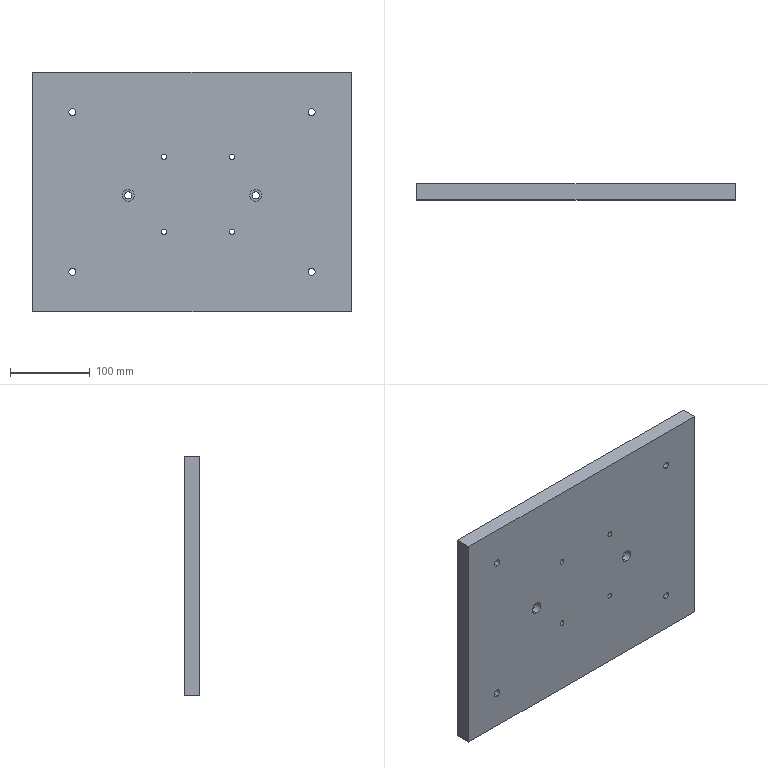Part | SolidWorks | features HoleWzd 3, Cut 1, Extrusion 1 | 1 solid | 50 faces | box 400 x 20 x 300 mm | volume 2382351 mm3 | cylinder 36 | plane 14 | commonest cylinder face diameters 9 x12 15 x12 6.8 x8 20 x4
STEP:
#1=CARTESIAN_POINT('',(-35.,0.,-53.4));
#2=VERTEX_POINT('',#1);
#3=CARTESIAN_POINT('',(-35.,0.,-46.6));
#4=VERTEX_POINT('',#3);
#5=CARTESIAN_POINT('',(-35.,0.,-50.));
#6=DIRECTION('',(0.,1.,0.));
#7=DIRECTION('',(0.,0.,1.));
#8=AXIS2_PLACEMENT_3D('',#5,#6,#7);
#9=CIRCLE('',#8,3.4);
#10=EDGE_CURVE('',#2,#4,#9,.T.);
#11=ORIENTED_EDGE('',*,*,#10,.F.);
#12=CARTESIAN_POINT('',(-35.,20.,-53.4));
#13=VERTEX_POINT('',#12);
#14=CARTESIAN_POINT('',(-35.,20.,-53.4));
#15=DIRECTION('',(0.,1.,0.));
#16=VECTOR('',#15,1000.);
#17=LINE('',#14,#16);
#18=EDGE_CURVE('',#2,#13,#17,.T.);
#19=ORIENTED_EDGE('',*,*,#18,.T.);
#20=CARTESIAN_POINT('',(-35.,20.,-46.6));
#21=VERTEX_POINT('',#20);
#22=CARTESIAN_POINT('',(-35.,20.,-50.));
#23=DIRECTION('',(0.,1.,0.));
#24=DIRECTION('',(0.,0.,1.));
#25=AXIS2_PLACEMENT_3D('',#22,#23,#24);
#26=CIRCLE('',#25,3.4);
#27=EDGE_CURVE('',#13,#21,#26,.T.);
#28=ORIENTED_EDGE('',*,*,#27,.T.);
#29=CARTESIAN_POINT('',(-35.,20.,-46.6));
#30=DIRECTION('',(0.,1.,0.));
#31=VECTOR('',#30,1000.);
#32=LINE('',#29,#31);
#33=EDGE_CURVE('',#4,#21,#32,.T.);
#34=ORIENTED_EDGE('',*,*,#33,.F.);
#35=EDGE_LOOP('',(#11,#19,#28,#34));
#36=FACE_OUTER_BOUND('',#35,.T.);
#37=CARTESIAN_POINT('',(-35.,20.,-50.));
#38=DIRECTION('',(0.,1.,0.));
#39=DIRECTION('',(0.,0.,1.));
#40=AXIS2_PLACEMENT_3D('',#37,#38,#39);
#41=CYLINDRICAL_SURFACE('',#40,3.4);
#42=ADVANCED_FACE('',(#36),#41,.F.);
#43=CARTESIAN_POINT('',(-35.,0.,40.6));
#44=VERTEX_POINT('',#43);
#45=CARTESIAN_POINT('',(-35.,0.,47.4));
#46=VERTEX_POINT('',#45);
#47=CARTESIAN_POINT('',(-35.,0.,44.));
#48=DIRECTION('',(0.,1.,0.));
#49=DIRECTION('',(0.,0.,1.));
#50=AXIS2_PLACEMENT_3D('',#47,#48,#49);
#51=CIRCLE('',#50,3.4);
#52=EDGE_CURVE('',#44,#46,#51,.T.);
#53=ORIENTED_EDGE('',*,*,#52,.F.);
#54=CARTESIAN_POINT('',(-35.,20.,40.6));
#55=VERTEX_POINT('',#54);
#56=CARTESIAN_POINT('',(-35.,20.,40.6));
#57=DIRECTION('',(0.,1.,0.));
#58=VECTOR('',#57,1000.);
#59=LINE('',#56,#58);
#60=EDGE_CURVE('',#44,#55,#59,.T.);
#61=ORIENTED_EDGE('',*,*,#60,.T.);
#62=CARTESIAN_POINT('',(-35.,20.,47.4));
#63=VERTEX_POINT('',#62);
#64=CARTESIAN_POINT('',(-35.,20.,44.));
#65=DIRECTION('',(0.,1.,0.));
#66=DIRECTION('',(0.,0.,1.));
#67=AXIS2_PLACEMENT_3D('',#64,#65,#66);
#68=CIRCLE('',#67,3.4);
#69=EDGE_CURVE('',#55,#63,#68,.T.);
#70=ORIENTED_EDGE('',*,*,#69,.T.);
#71=CARTESIAN_POINT('',(-35.,20.,47.4));
#72=DIRECTION('',(0.,1.,0.));
#73=VECTOR('',#72,1000.);
#74=LINE('',#71,#73);
#75=EDGE_CURVE('',#46,#63,#74,.T.);
#76=ORIENTED_EDGE('',*,*,#75,.F.);
#77=EDGE_LOOP('',(#53,#61,#70,#76));
#78=FACE_OUTER_BOUND('',#77,.T.);
#79=CARTESIAN_POINT('',(-35.,20.,44.));
#80=DIRECTION('',(0.,1.,0.));
#81=DIRECTION('',(0.,0.,1.));
#82=AXIS2_PLACEMENT_3D('',#79,#80,#81);
#83=CYLINDRICAL_SURFACE('',#82,3.4);
#84=ADVANCED_FACE('',(#78),#83,.F.);
#85=CARTESIAN_POINT('',(50.,0.,40.6));
#86=VERTEX_POINT('',#85);
#87=CARTESIAN_POINT('',(50.,0.,47.4));
#88=VERTEX_POINT('',#87);
#89=CARTESIAN_POINT('',(50.,0.,44.));
#90=DIRECTION('',(0.,1.,0.));
#91=DIRECTION('',(0.,0.,1.));
#92=AXIS2_PLACEMENT_3D('',#89,#90,#91);
#93=CIRCLE('',#92,3.4);
#94=EDGE_CURVE('',#86,#88,#93,.T.);
#95=ORIENTED_EDGE('',*,*,#94,.F.);
#96=CARTESIAN_POINT('',(50.,20.,40.6));
#97=VERTEX_POINT('',#96);
#98=CARTESIAN_POINT('',(50.,20.,40.6));
#99=DIRECTION('',(0.,1.,0.));
#100=VECTOR('',#99,1000.);
#101=LINE('',#98,#100);
#102=EDGE_CURVE('',#86,#97,#101,.T.);
#103=ORIENTED_EDGE('',*,*,#102,.T.);
#104=CARTESIAN_POINT('',(50.,20.,47.4));
#105=VERTEX_POINT('',#104);
#106=CARTESIAN_POINT('',(50.,20.,44.));
#107=DIRECTION('',(0.,1.,0.));
#108=DIRECTION('',(0.,0.,1.));
#109=AXIS2_PLACEMENT_3D('',#106,#107,#108);
#110=CIRCLE('',#109,3.4);
#111=EDGE_CURVE('',#97,#105,#110,.T.);
#112=ORIENTED_EDGE('',*,*,#111,.T.);
#113=CARTESIAN_POINT('',(50.,20.,47.4));
#114=DIRECTION('',(0.,1.,0.));
#115=VECTOR('',#114,1000.);
#116=LINE('',#113,#115);
#117=EDGE_CURVE('',#88,#105,#116,.T.);
#118=ORIENTED_EDGE('',*,*,#117,.F.);
#119=EDGE_LOOP('',(#95,#103,#112,#118));
#120=FACE_OUTER_BOUND('',#119,.T.);
#121=CARTESIAN_POINT('',(50.,20.,44.));
#122=DIRECTION('',(0.,1.,0.));
#123=DIRECTION('',(0.,0.,1.));
#124=AXIS2_PLACEMENT_3D('',#121,#122,#123);
#125=CYLINDRICAL_SURFACE('',#124,3.4);
#126=ADVANCED_FACE('',(#120),#125,.F.);
#127=CARTESIAN_POINT('',(50.,0.,-53.4));
#128=VERTEX_POINT('',#127);
#129=CARTESIAN_POINT('',(50.,0.,-46.6));
#130=VERTEX_POINT('',#129);
#131=CARTESIAN_POINT('',(50.,0.,-50.));
#132=DIRECTION('',(0.,1.,0.));
#133=DIRECTION('',(0.,0.,1.));
#134=AXIS2_PLACEMENT_3D('',#131,#132,#133);
#135=CIRCLE('',#134,3.4);
#136=EDGE_CURVE('',#128,#130,#135,.T.);
#137=ORIENTED_EDGE('',*,*,#136,.F.);
#138=CARTESIAN_POINT('',(50.,20.,-53.4));
#139=VERTEX_POINT('',#138);
#140=CARTESIAN_POINT('',(50.,20.,-53.4));
#141=DIRECTION('',(0.,1.,0.));
#142=VECTOR('',#141,1000.);
#143=LINE('',#140,#142);
#144=EDGE_CURVE('',#128,#139,#143,.T.);
#145=ORIENTED_EDGE('',*,*,#144,.T.);
#146=CARTESIAN_POINT('',(50.,20.,-46.6));
#147=VERTEX_POINT('',#146);
#148=CARTESIAN_POINT('',(50.,20.,-50.));
#149=DIRECTION('',(0.,1.,0.));
#150=DIRECTION('',(0.,0.,1.));
#151=AXIS2_PLACEMENT_3D('',#148,#149,#150);
#152=CIRCLE('',#151,3.4);
#153=EDGE_CURVE('',#139,#147,#152,.T.);
#154=ORIENTED_EDGE('',*,*,#153,.T.);
#155=CARTESIAN_POINT('',(50.,20.,-46.6));
#156=DIRECTION('',(0.,1.,0.));
#157=VECTOR('',#156,1000.);
#158=LINE('',#155,#157);
#159=EDGE_CURVE('',#130,#147,#158,.T.);
#160=ORIENTED_EDGE('',*,*,#159,.F.);
#161=EDGE_LOOP('',(#137,#145,#154,#160));
#162=FACE_OUTER_BOUND('',#161,.T.);
#163=CARTESIAN_POINT('',(50.,20.,-50.));
#164=DIRECTION('',(0.,1.,0.));
#165=DIRECTION('',(0.,0.,1.));
#166=AXIS2_PLACEMENT_3D('',#163,#164,#165);
#167=CYLINDRICAL_SURFACE('',#166,3.4);
#168=ADVANCED_FACE('',(#162),#167,.F.);
#169=CARTESIAN_POINT('',(-80.,9.,3.334));
#170=VERTEX_POINT('',#169);
#171=CARTESIAN_POINT('',(-80.,9.,-11.666));
#172=VERTEX_POINT('',#171);
#173=CARTESIAN_POINT('',(-80.,9.,-4.166));
#174=DIRECTION('',(0.,-1.,0.));
#175=DIRECTION('',(0.,0.,-1.));
#176=AXIS2_PLACEMENT_3D('',#173,#174,#175);
#177=CIRCLE('',#176,7.5);
#178=EDGE_CURVE('',#170,#172,#177,.T.);
#179=ORIENTED_EDGE('',*,*,#178,.F.);
#180=CARTESIAN_POINT('',(-80.,0.,3.334));
#181=VERTEX_POINT('',#180);
#182=CARTESIAN_POINT('',(-80.,0.,3.334));
#183=DIRECTION('',(0.,-1.,0.));
#184=VECTOR('',#183,1000.);
#185=LINE('',#182,#184);
#186=EDGE_CURVE('',#170,#181,#185,.T.);
#187=ORIENTED_EDGE('',*,*,#186,.T.);
#188=CARTESIAN_POINT('',(-80.,0.,-11.666));
#189=VERTEX_POINT('',#188);
#190=CARTESIAN_POINT('',(-80.,0.,-4.166));
#191=DIRECTION('',(0.,-1.,0.));
#192=DIRECTION('',(0.,0.,-1.));
#193=AXIS2_PLACEMENT_3D('',#190,#191,#192);
#194=CIRCLE('',#193,7.5);
#195=EDGE_CURVE('',#181,#189,#194,.T.);
#196=ORIENTED_EDGE('',*,*,#195,.T.);
#197=CARTESIAN_POINT('',(-80.,0.,-11.666));
#198=DIRECTION('',(0.,-1.,0.));
#199=VECTOR('',#198,1000.);
#200=LINE('',#197,#199);
#201=EDGE_CURVE('',#172,#189,#200,.T.);
#202=ORIENTED_EDGE('',*,*,#201,.F.);
#203=EDGE_LOOP('',(#179,#187,#196,#202));
#204=FACE_OUTER_BOUND('',#203,.T.);
#205=CARTESIAN_POINT('',(-80.,0.,-4.166));
#206=DIRECTION('',(0.,-1.,0.));
#207=DIRECTION('',(0.,0.,-1.));
#208=AXIS2_PLACEMENT_3D('',#205,#206,#207);
#209=CYLINDRICAL_SURFACE('',#208,7.5);
#210=ADVANCED_FACE('',(#204),#209,.F.);
#211=CARTESIAN_POINT('',(-80.,18.,-8.666));
#212=VERTEX_POINT('',#211);
#213=CARTESIAN_POINT('',(-80.,18.,0.3336));
#214=VERTEX_POINT('',#213);
#215=CARTESIAN_POINT('',(-80.,18.,-4.166));
#216=DIRECTION('',(0.,1.,0.));
#217=DIRECTION('',(0.,0.,1.));
#218=AXIS2_PLACEMENT_3D('',#215,#216,#217);
#219=CIRCLE('',#218,4.5);
#220=EDGE_CURVE('',#212,#214,#219,.T.);
#221=ORIENTED_EDGE('',*,*,#220,.T.);
#222=CARTESIAN_POINT('',(-80.,9.,0.3336));
#223=VERTEX_POINT('',#222);
#224=CARTESIAN_POINT('',(-80.,0.,0.3336));
#225=DIRECTION('',(0.,-1.,0.));
#226=VECTOR('',#225,1000.);
#227=LINE('',#224,#226);
#228=EDGE_CURVE('',#214,#223,#227,.T.);
#229=ORIENTED_EDGE('',*,*,#228,.T.);
#230=CARTESIAN_POINT('',(-80.,9.,-8.666));
#231=VERTEX_POINT('',#230);
#232=CARTESIAN_POINT('',(-80.,9.,-4.166));
#233=DIRECTION('',(0.,-1.,0.));
#234=DIRECTION('',(0.,0.,-1.));
#235=AXIS2_PLACEMENT_3D('',#232,#233,#234);
#236=CIRCLE('',#235,4.5);
#237=EDGE_CURVE('',#223,#231,#236,.T.);
#238=ORIENTED_EDGE('',*,*,#237,.T.);
#239=CARTESIAN_POINT('',(-80.,0.,-8.666));
#240=DIRECTION('',(0.,-1.,0.));
#241=VECTOR('',#240,1000.);
#242=LINE('',#239,#241);
#243=EDGE_CURVE('',#212,#231,#242,.T.);
#244=ORIENTED_EDGE('',*,*,#243,.F.);
#245=EDGE_LOOP('',(#221,#229,#238,#244));
#246=FACE_OUTER_BOUND('',#245,.T.);
#247=CARTESIAN_POINT('',(-80.,0.,-4.166));
#248=DIRECTION('',(0.,-1.,0.));
#249=DIRECTION('',(0.,0.,-1.));
#250=AXIS2_PLACEMENT_3D('',#247,#248,#249);
#251=CYLINDRICAL_SURFACE('',#250,4.5);
#252=ADVANCED_FACE('',(#246),#251,.F.);
#253=CARTESIAN_POINT('',(80.,9.,3.334));
#254=VERTEX_POINT('',#253);
#255=CARTESIAN_POINT('',(80.,9.,-11.666));
#256=VERTEX_POINT('',#255);
#257=CARTESIAN_POINT('',(80.,9.,-4.166));
#258=DIRECTION('',(0.,-1.,0.));
#259=DIRECTION('',(0.,0.,-1.));
#260=AXIS2_PLACEMENT_3D('',#257,#258,#259);
#261=CIRCLE('',#260,7.5);
#262=EDGE_CURVE('',#254,#256,#261,.T.);
#263=ORIENTED_EDGE('',*,*,#262,.F.);
#264=CARTESIAN_POINT('',(80.,0.,3.334));
#265=VERTEX_POINT('',#264);
#266=CARTESIAN_POINT('',(80.,0.,3.334));
#267=DIRECTION('',(0.,-1.,0.));
#268=VECTOR('',#267,1000.);
#269=LINE('',#266,#268);
#270=EDGE_CURVE('',#254,#265,#269,.T.);
#271=ORIENTED_EDGE('',*,*,#270,.T.);
#272=CARTESIAN_POINT('',(80.,0.,-11.666));
#273=VERTEX_POINT('',#272);
#274=CARTESIAN_POINT('',(80.,0.,-4.166));
#275=DIRECTION('',(0.,-1.,0.));
#276=DIRECTION('',(0.,0.,-1.));
#277=AXIS2_PLACEMENT_3D('',#274,#275,#276);
#278=CIRCLE('',#277,7.5);
#279=EDGE_CURVE('',#265,#273,#278,.T.);
#280=ORIENTED_EDGE('',*,*,#279,.T.);
#281=CARTESIAN_POINT('',(80.,0.,-11.666));
#282=DIRECTION('',(0.,-1.,0.));
#283=VECTOR('',#282,1000.);
#284=LINE('',#281,#283);
#285=EDGE_CURVE('',#256,#273,#284,.T.);
#286=ORIENTED_EDGE('',*,*,#285,.F.);
#287=EDGE_LOOP('',(#263,#271,#280,#286));
#288=FACE_OUTER_BOUND('',#287,.T.);
#289=CARTESIAN_POINT('',(80.,0.,-4.166));
#290=DIRECTION('',(0.,-1.,0.));
#291=DIRECTION('',(0.,0.,-1.));
#292=AXIS2_PLACEMENT_3D('',#289,#290,#291);
#293=CYLINDRICAL_SURFACE('',#292,7.5);
#294=ADVANCED_FACE('',(#288),#293,.F.);
#295=CARTESIAN_POINT('',(80.,18.,-8.666));
#296=VERTEX_POINT('',#295);
#297=CARTESIAN_POINT('',(80.,18.,0.3336));
#298=VERTEX_POINT('',#297);
#299=CARTESIAN_POINT('',(80.,18.,-4.166));
#300=DIRECTION('',(0.,1.,0.));
#301=DIRECTION('',(0.,0.,1.));
#302=AXIS2_PLACEMENT_3D('',#299,#300,#301);
#303=CIRCLE('',#302,4.5);
#304=EDGE_CURVE('',#296,#298,#303,.T.);
#305=ORIENTED_EDGE('',*,*,#304,.T.);
#306=CARTESIAN_POINT('',(80.,9.,0.3336));
#307=VERTEX_POINT('',#306);
#308=CARTESIAN_POINT('',(80.,0.,0.3336));
#309=DIRECTION('',(0.,-1.,0.));
#310=VECTOR('',#309,1000.);
#311=LINE('',#308,#310);
#312=EDGE_CURVE('',#298,#307,#311,.T.);
#313=ORIENTED_EDGE('',*,*,#312,.T.);
#314=CARTESIAN_POINT('',(80.,9.,-8.666));
#315=VERTEX_POINT('',#314);
#316=CARTESIAN_POINT('',(80.,9.,-4.166));
#317=DIRECTION('',(0.,-1.,0.));
#318=DIRECTION('',(0.,0.,-1.));
#319=AXIS2_PLACEMENT_3D('',#316,#317,#318);
#320=CIRCLE('',#319,4.5);
#321=EDGE_CURVE('',#307,#315,#320,.T.);
#322=ORIENTED_EDGE('',*,*,#321,.T.);
#323=CARTESIAN_POINT('',(80.,0.,-8.666));
#324=DIRECTION('',(0.,-1.,0.));
#325=VECTOR('',#324,1000.);
#326=LINE('',#323,#325);
#327=EDGE_CURVE('',#296,#315,#326,.T.);
#328=ORIENTED_EDGE('',*,*,#327,.F.);
#329=EDGE_LOOP('',(#305,#313,#322,#328));
#330=FACE_OUTER_BOUND('',#329,.T.);
#331=CARTESIAN_POINT('',(80.,0.,-4.166));
#332=DIRECTION('',(0.,-1.,0.));
#333=DIRECTION('',(0.,0.,-1.));
#334=AXIS2_PLACEMENT_3D('',#331,#332,#333);
#335=CYLINDRICAL_SURFACE('',#334,4.5);
#336=ADVANCED_FACE('',(#330),#335,.F.);
#337=CARTESIAN_POINT('',(-80.,18.,-14.166));
#338=VERTEX_POINT('',#337);
#339=CARTESIAN_POINT('',(-80.,18.,5.834));
#340=VERTEX_POINT('',#339);
#341=CARTESIAN_POINT('',(-80.,18.,-4.166));
#342=DIRECTION('',(0.,1.,0.));
#343=DIRECTION('',(0.,0.,1.));
#344=AXIS2_PLACEMENT_3D('',#341,#342,#343);
#345=CIRCLE('',#344,10.);
#346=EDGE_CURVE('',#338,#340,#345,.T.);
#347=ORIENTED_EDGE('',*,*,#346,.F.);
#348=CARTESIAN_POINT('',(-80.,20.,-14.166));
#349=VERTEX_POINT('',#348);
#350=CARTESIAN_POINT('',(-80.,18.,-14.166));
#351=DIRECTION('',(0.,1.,0.));
#352=VECTOR('',#351,1000.);
#353=LINE('',#350,#352);
#354=EDGE_CURVE('',#338,#349,#353,.T.);
#355=ORIENTED_EDGE('',*,*,#354,.T.);
#356=CARTESIAN_POINT('',(-80.,20.,5.834));
#357=VERTEX_POINT('',#356);
#358=CARTESIAN_POINT('',(-80.,20.,-4.166));
#359=DIRECTION('',(0.,1.,0.));
#360=DIRECTION('',(0.,0.,1.));
#361=AXIS2_PLACEMENT_3D('',#358,#359,#360);
#362=CIRCLE('',#361,10.);
#363=EDGE_CURVE('',#349,#357,#362,.T.);
#364=ORIENTED_EDGE('',*,*,#363,.T.);
#365=CARTESIAN_POINT('',(-80.,18.,5.834));
#366=DIRECTION('',(0.,1.,0.));
#367=VECTOR('',#366,1000.);
#368=LINE('',#365,#367);
#369=EDGE_CURVE('',#340,#357,#368,.T.);
#370=ORIENTED_EDGE('',*,*,#369,.F.);
#371=EDGE_LOOP('',(#347,#355,#364,#370));
#372=FACE_OUTER_BOUND('',#371,.T.);
#373=CARTESIAN_POINT('',(-80.,18.,-4.166));
#374=DIRECTION('',(0.,1.,0.));
#375=DIRECTION('',(0.,0.,1.));
#376=AXIS2_PLACEMENT_3D('',#373,#374,#375);
#377=CYLINDRICAL_SURFACE('',#376,10.);
#378=ADVANCED_FACE('',(#372),#377,.F.);
#379=CARTESIAN_POINT('',(80.,18.,-14.166));
#380=VERTEX_POINT('',#379);
#381=CARTESIAN_POINT('',(80.,18.,5.834));
#382=VERTEX_POINT('',#381);
#383=CARTESIAN_POINT('',(80.,18.,-4.166));
#384=DIRECTION('',(0.,1.,0.));
#385=DIRECTION('',(0.,0.,1.));
#386=AXIS2_PLACEMENT_3D('',#383,#384,#385);
#387=CIRCLE('',#386,10.);
#388=EDGE_CURVE('',#380,#382,#387,.T.);
#389=ORIENTED_EDGE('',*,*,#388,.F.);
#390=CARTESIAN_POINT('',(80.,20.,-14.166));
#391=VERTEX_POINT('',#390);
#392=CARTESIAN_POINT('',(80.,18.,-14.166));
#393=DIRECTION('',(0.,1.,0.));
#394=VECTOR('',#393,1000.);
#395=LINE('',#392,#394);
#396=EDGE_CURVE('',#380,#391,#395,.T.);
#397=ORIENTED_EDGE('',*,*,#396,.T.);
#398=CARTESIAN_POINT('',(80.,20.,5.834));
#399=VERTEX_POINT('',#398);
#400=CARTESIAN_POINT('',(80.,20.,-4.166));
#401=DIRECTION('',(0.,1.,0.));
#402=DIRECTION('',(0.,0.,1.));
#403=AXIS2_PLACEMENT_3D('',#400,#401,#402);
#404=CIRCLE('',#403,10.);
#405=EDGE_CURVE('',#391,#399,#404,.T.);
#406=ORIENTED_EDGE('',*,*,#405,.T.);
#407=CARTESIAN_POINT('',(80.,18.,5.834));
#408=DIRECTION('',(0.,1.,0.));
#409=VECTOR('',#408,1000.);
#410=LINE('',#407,#409);
#411=EDGE_CURVE('',#382,#399,#410,.T.);
#412=ORIENTED_EDGE('',*,*,#411,.F.);
#413=EDGE_LOOP('',(#389,#397,#406,#412));
#414=FACE_OUTER_BOUND('',#413,.T.);
#415=CARTESIAN_POINT('',(80.,18.,-4.166));
#416=DIRECTION('',(0.,1.,0.));
#417=DIRECTION('',(0.,0.,1.));
#418=AXIS2_PLACEMENT_3D('',#415,#416,#417);
#419=CYLINDRICAL_SURFACE('',#418,10.);
#420=ADVANCED_FACE('',(#414),#419,.F.);
#421=CARTESIAN_POINT('',(-150.,11.,-107.5));
#422=VERTEX_POINT('',#421);
#423=CARTESIAN_POINT('',(-150.,11.,-92.5));
#424=VERTEX_POINT('',#423);
#425=CARTESIAN_POINT('',(-150.,11.,-100.));
#426=DIRECTION('',(0.,1.,0.));
#427=DIRECTION('',(0.,0.,1.));
#428=AXIS2_PLACEMENT_3D('',#425,#426,#427);
#429=CIRCLE('',#428,7.5);
#430=EDGE_CURVE('',#422,#424,#429,.T.);
#431=ORIENTED_EDGE('',*,*,#430,.F.);
#432=CARTESIAN_POINT('',(-150.,20.,-107.5));
#433=VERTEX_POINT('',#432);
#434=CARTESIAN_POINT('',(-150.,20.,-107.5));
#435=DIRECTION('',(0.,1.,0.));
#436=VECTOR('',#435,1000.);
#437=LINE('',#434,#436);
#438=EDGE_CURVE('',#422,#433,#437,.T.);
#439=ORIENTED_EDGE('',*,*,#438,.T.);
#440=CARTESIAN_POINT('',(-150.,20.,-92.5));
#441=VERTEX_POINT('',#440);
#442=CARTESIAN_POINT('',(-150.,20.,-100.));
#443=DIRECTION('',(0.,1.,0.));
#444=DIRECTION('',(0.,0.,1.));
#445=AXIS2_PLACEMENT_3D('',#442,#443,#444);
#446=CIRCLE('',#445,7.5);
#447=EDGE_CURVE('',#433,#441,#446,.T.);
#448=ORIENTED_EDGE('',*,*,#447,.T.);
#449=CARTESIAN_POINT('',(-150.,20.,-92.5));
#450=DIRECTION('',(0.,1.,0.));
#451=VECTOR('',#450,1000.);
#452=LINE('',#449,#451);
#453=EDGE_CURVE('',#424,#441,#452,.T.);
#454=ORIENTED_EDGE('',*,*,#453,.F.);
#455=EDGE_LOOP('',(#431,#439,#448,#454));
#456=FACE_OUTER_BOUND('',#455,.T.);
#457=CARTESIAN_POINT('',(-150.,20.,-100.));
#458=DIRECTION('',(0.,1.,0.));
#459=DIRECTION('',(0.,0.,1.));
#460=AXIS2_PLACEMENT_3D('',#457,#458,#459);
#461=CYLINDRICAL_SURFACE('',#460,7.5);
#462=ADVANCED_FACE('',(#456),#461,.F.);
#463=CARTESIAN_POINT('',(-150.,0.,-104.5));
#464=VERTEX_POINT('',#463);
#465=CARTESIAN_POINT('',(-150.,0.,-95.5));
#466=VERTEX_POINT('',#465);
#467=CARTESIAN_POINT('',(-150.,0.,-100.));
#468=DIRECTION('',(0.,1.,0.));
#469=DIRECTION('',(0.,0.,1.));
#470=AXIS2_PLACEMENT_3D('',#467,#468,#469);
#471=CIRCLE('',#470,4.5);
#472=EDGE_CURVE('',#464,#466,#471,.T.);
#473=ORIENTED_EDGE('',*,*,#472,.F.);
#474=CARTESIAN_POINT('',(-150.,11.,-104.5));
#475=VERTEX_POINT('',#474);
#476=CARTESIAN_POINT('',(-150.,20.,-104.5));
#477=DIRECTION('',(0.,1.,0.));
#478=VECTOR('',#477,1000.);
#479=LINE('',#476,#478);
#480=EDGE_CURVE('',#464,#475,#479,.T.);
#481=ORIENTED_EDGE('',*,*,#480,.T.);
#482=CARTESIAN_POINT('',(-150.,11.,-95.5));
#483=VERTEX_POINT('',#482);
#484=CARTESIAN_POINT('',(-150.,11.,-100.));
#485=DIRECTION('',(0.,1.,0.));
#486=DIRECTION('',(0.,0.,1.));
#487=AXIS2_PLACEMENT_3D('',#484,#485,#486);
#488=CIRCLE('',#487,4.5);
#489=EDGE_CURVE('',#475,#483,#488,.T.);
#490=ORIENTED_EDGE('',*,*,#489,.T.);
#491=CARTESIAN_POINT('',(-150.,20.,-95.5));
#492=DIRECTION('',(0.,1.,0.));
#493=VECTOR('',#492,1000.);
#494=LINE('',#491,#493);
#495=EDGE_CURVE('',#466,#483,#494,.T.);
#496=ORIENTED_EDGE('',*,*,#495,.F.);
#497=EDGE_LOOP('',(#473,#481,#490,#496));
#498=FACE_OUTER_BOUND('',#497,.T.);
#499=CARTESIAN_POINT('',(-150.,20.,-100.));
#500=DIRECTION('',(0.,1.,0.));
#501=DIRECTION('',(0.,0.,1.));
#502=AXIS2_PLACEMENT_3D('',#499,#500,#501);
#503=CYLINDRICAL_SURFACE('',#502,4.5);
#504=ADVANCED_FACE('',(#498),#503,.F.);
#505=CARTESIAN_POINT('',(-150.,11.,92.5));
#506=VERTEX_POINT('',#505);
#507=CARTESIAN_POINT('',(-150.,11.,107.5));
#508=VERTEX_POINT('',#507);
#509=CARTESIAN_POINT('',(-150.,11.,100.));
#510=DIRECTION('',(0.,1.,0.));
#511=DIRECTION('',(0.,0.,1.));
#512=AXIS2_PLACEMENT_3D('',#509,#510,#511);
#513=CIRCLE('',#512,7.5);
#514=EDGE_CURVE('',#506,#508,#513,.T.);
#515=ORIENTED_EDGE('',*,*,#514,.F.);
#516=CARTESIAN_POINT('',(-150.,20.,92.5));
#517=VERTEX_POINT('',#516);
#518=CARTESIAN_POINT('',(-150.,20.,92.5));
#519=DIRECTION('',(0.,1.,0.));
#520=VECTOR('',#519,1000.);
#521=LINE('',#518,#520);
#522=EDGE_CURVE('',#506,#517,#521,.T.);
#523=ORIENTED_EDGE('',*,*,#522,.T.);
#524=CARTESIAN_POINT('',(-150.,20.,107.5));
#525=VERTEX_POINT('',#524);
#526=CARTESIAN_POINT('',(-150.,20.,100.));
#527=DIRECTION('',(0.,1.,0.));
#528=DIRECTION('',(0.,0.,1.));
#529=AXIS2_PLACEMENT_3D('',#526,#527,#528);
#530=CIRCLE('',#529,7.5);
#531=EDGE_CURVE('',#517,#525,#530,.T.);
#532=ORIENTED_EDGE('',*,*,#531,.T.);
#533=CARTESIAN_POINT('',(-150.,20.,107.5));
#534=DIRECTION('',(0.,1.,0.));
#535=VECTOR('',#534,1000.);
#536=LINE('',#533,#535);
#537=EDGE_CURVE('',#508,#525,#536,.T.);
#538=ORIENTED_EDGE('',*,*,#537,.F.);
#539=EDGE_LOOP('',(#515,#523,#532,#538));
#540=FACE_OUTER_BOUND('',#539,.T.);
#541=CARTESIAN_POINT('',(-150.,20.,100.));
#542=DIRECTION('',(0.,1.,0.));
#543=DIRECTION('',(0.,0.,1.));
#544=AXIS2_PLACEMENT_3D('',#541,#542,#543);
#545=CYLINDRICAL_SURFACE('',#544,7.5);
#546=ADVANCED_FACE('',(#540),#545,.F.);
#547=CARTESIAN_POINT('',(-150.,0.,95.5));
#548=VERTEX_POINT('',#547);
#549=CARTESIAN_POINT('',(-150.,0.,104.5));
#550=VERTEX_POINT('',#549);
#551=CARTESIAN_POINT('',(-150.,0.,100.));
#552=DIRECTION('',(0.,1.,0.));
#553=DIRECTION('',(0.,0.,1.));
#554=AXIS2_PLACEMENT_3D('',#551,#552,#553);
#555=CIRCLE('',#554,4.5);
#556=EDGE_CURVE('',#548,#550,#555,.T.);
#557=ORIENTED_EDGE('',*,*,#556,.F.);
#558=CARTESIAN_POINT('',(-150.,11.,95.5));
#559=VERTEX_POINT('',#558);
#560=CARTESIAN_POINT('',(-150.,20.,95.5));
#561=DIRECTION('',(0.,1.,0.));
#562=VECTOR('',#561,1000.);
#563=LINE('',#560,#562);
#564=EDGE_CURVE('',#548,#559,#563,.T.);
#565=ORIENTED_EDGE('',*,*,#564,.T.);
#566=CARTESIAN_POINT('',(-150.,11.,104.5));
#567=VERTEX_POINT('',#566);
#568=CARTESIAN_POINT('',(-150.,11.,100.));
#569=DIRECTION('',(0.,1.,0.));
#570=DIRECTION('',(0.,0.,1.));
#571=AXIS2_PLACEMENT_3D('',#568,#569,#570);
#572=CIRCLE('',#571,4.5);
#573=EDGE_CURVE('',#559,#567,#572,.T.);
#574=ORIENTED_EDGE('',*,*,#573,.T.);
#575=CARTESIAN_POINT('',(-150.,20.,104.5));
#576=DIRECTION('',(0.,1.,0.));
#577=VECTOR('',#576,1000.);
#578=LINE('',#575,#577);
#579=EDGE_CURVE('',#550,#567,#578,.T.);
#580=ORIENTED_EDGE('',*,*,#579,.F.);
#581=EDGE_LOOP('',(#557,#565,#574,#580));
#582=FACE_OUTER_BOUND('',#581,.T.);
#583=CARTESIAN_POINT('',(-150.,20.,100.));
#584=DIRECTION('',(0.,1.,0.));
#585=DIRECTION('',(0.,0.,1.));
#586=AXIS2_PLACEMENT_3D('',#583,#584,#585);
#587=CYLINDRICAL_SURFACE('',#586,4.5);
#588=ADVANCED_FACE('',(#582),#587,.F.);
#589=CARTESIAN_POINT('',(150.,11.,-107.5));
#590=VERTEX_POINT('',#589);
#591=CARTESIAN_POINT('',(150.,11.,-92.5));
#592=VERTEX_POINT('',#591);
#593=CARTESIAN_POINT('',(150.,11.,-100.));
#594=DIRECTION('',(0.,1.,0.));
#595=DIRECTION('',(0.,0.,1.));
#596=AXIS2_PLACEMENT_3D('',#593,#594,#595);
#597=CIRCLE('',#596,7.5);
#598=EDGE_CURVE('',#590,#592,#597,.T.);
#599=ORIENTED_EDGE('',*,*,#598,.F.);
#600=CARTESIAN_POINT('',(150.,20.,-107.5));
#601=VERTEX_POINT('',#600);
#602=CARTESIAN_POINT('',(150.,20.,-107.5));
#603=DIRECTION('',(0.,1.,0.));
#604=VECTOR('',#603,1000.);
#605=LINE('',#602,#604);
#606=EDGE_CURVE('',#590,#601,#605,.T.);
#607=ORIENTED_EDGE('',*,*,#606,.T.);
#608=CARTESIAN_POINT('',(150.,20.,-92.5));
#609=VERTEX_POINT('',#608);
#610=CARTESIAN_POINT('',(150.,20.,-100.));
#611=DIRECTION('',(0.,1.,0.));
#612=DIRECTION('',(0.,0.,1.));
#613=AXIS2_PLACEMENT_3D('',#610,#611,#612);
#614=CIRCLE('',#613,7.5);
#615=EDGE_CURVE('',#601,#609,#614,.T.);
#616=ORIENTED_EDGE('',*,*,#615,.T.);
#617=CARTESIAN_POINT('',(150.,20.,-92.5));
#618=DIRECTION('',(0.,1.,0.));
#619=VECTOR('',#618,1000.);
#620=LINE('',#617,#619);
#621=EDGE_CURVE('',#592,#609,#620,.T.);
#622=ORIENTED_EDGE('',*,*,#621,.F.);
#623=EDGE_LOOP('',(#599,#607,#616,#622));
#624=FACE_OUTER_BOUND('',#623,.T.);
#625=CARTESIAN_POINT('',(150.,20.,-100.));
#626=DIRECTION('',(0.,1.,0.));
#627=DIRECTION('',(0.,0.,1.));
#628=AXIS2_PLACEMENT_3D('',#625,#626,#627);
#629=CYLINDRICAL_SURFACE('',#628,7.5);
#630=ADVANCED_FACE('',(#624),#629,.F.);
#631=CARTESIAN_POINT('',(150.,0.,-104.5));
#632=VERTEX_POINT('',#631);
#633=CARTESIAN_POINT('',(150.,0.,-95.5));
#634=VERTEX_POINT('',#633);
#635=CARTESIAN_POINT('',(150.,0.,-100.));
#636=DIRECTION('',(0.,1.,0.));
#637=DIRECTION('',(0.,0.,1.));
#638=AXIS2_PLACEMENT_3D('',#635,#636,#637);
#639=CIRCLE('',#638,4.5);
#640=EDGE_CURVE('',#632,#634,#639,.T.);
#641=ORIENTED_EDGE('',*,*,#640,.F.);
#642=CARTESIAN_POINT('',(150.,11.,-104.5));
#643=VERTEX_POINT('',#642);
#644=CARTESIAN_POINT('',(150.,20.,-104.5));
#645=DIRECTION('',(0.,1.,0.));
#646=VECTOR('',#645,1000.);
#647=LINE('',#644,#646);
#648=EDGE_CURVE('',#632,#643,#647,.T.);
#649=ORIENTED_EDGE('',*,*,#648,.T.);
#650=CARTESIAN_POINT('',(150.,11.,-95.5));
#651=VERTEX_POINT('',#650);
#652=CARTESIAN_POINT('',(150.,11.,-100.));
#653=DIRECTION('',(0.,1.,0.));
#654=DIRECTION('',(0.,0.,1.));
#655=AXIS2_PLACEMENT_3D('',#652,#653,#654);
#656=CIRCLE('',#655,4.5);
#657=EDGE_CURVE('',#643,#651,#656,.T.);
#658=ORIENTED_EDGE('',*,*,#657,.T.);
#659=CARTESIAN_POINT('',(150.,20.,-95.5));
#660=DIRECTION('',(0.,1.,0.));
#661=VECTOR('',#660,1000.);
#662=LINE('',#659,#661);
#663=EDGE_CURVE('',#634,#651,#662,.T.);
#664=ORIENTED_EDGE('',*,*,#663,.F.);
#665=EDGE_LOOP('',(#641,#649,#658,#664));
#666=FACE_OUTER_BOUND('',#665,.T.);
#667=CARTESIAN_POINT('',(150.,20.,-100.));
#668=DIRECTION('',(0.,1.,0.));
#669=DIRECTION('',(0.,0.,1.));
#670=AXIS2_PLACEMENT_3D('',#667,#668,#669);
#671=CYLINDRICAL_SURFACE('',#670,4.5);
#672=ADVANCED_FACE('',(#666),#671,.F.);
#673=CARTESIAN_POINT('',(150.,11.,92.5));
#674=VERTEX_POINT('',#673);
#675=CARTESIAN_POINT('',(150.,11.,107.5));
#676=VERTEX_POINT('',#675);
#677=CARTESIAN_POINT('',(150.,11.,100.));
#678=DIRECTION('',(0.,1.,0.));
#679=DIRECTION('',(0.,0.,1.));
#680=AXIS2_PLACEMENT_3D('',#677,#678,#679);
#681=CIRCLE('',#680,7.5);
#682=EDGE_CURVE('',#674,#676,#681,.T.);
#683=ORIENTED_EDGE('',*,*,#682,.F.);
#684=CARTESIAN_POINT('',(150.,20.,92.5));
#685=VERTEX_POINT('',#684);
#686=CARTESIAN_POINT('',(150.,20.,92.5));
#687=DIRECTION('',(0.,1.,0.));
#688=VECTOR('',#687,1000.);
#689=LINE('',#686,#688);
#690=EDGE_CURVE('',#674,#685,#689,.T.);
#691=ORIENTED_EDGE('',*,*,#690,.T.);
#692=CARTESIAN_POINT('',(150.,20.,107.5));
#693=VERTEX_POINT('',#692);
#694=CARTESIAN_POINT('',(150.,20.,100.));
#695=DIRECTION('',(0.,1.,0.));
#696=DIRECTION('',(0.,0.,1.));
#697=AXIS2_PLACEMENT_3D('',#694,#695,#696);
#698=CIRCLE('',#697,7.5);
#699=EDGE_CURVE('',#685,#693,#698,.T.);
#700=ORIENTED_EDGE('',*,*,#699,.T.);
#701=CARTESIAN_POINT('',(150.,20.,107.5));
#702=DIRECTION('',(0.,1.,0.));
#703=VECTOR('',#702,1000.);
#704=LINE('',#701,#703);
#705=EDGE_CURVE('',#676,#693,#704,.T.);
#706=ORIENTED_EDGE('',*,*,#705,.F.);
#707=EDGE_LOOP('',(#683,#691,#700,#706));
#708=FACE_OUTER_BOUND('',#707,.T.);
#709=CARTESIAN_POINT('',(150.,20.,100.));
#710=DIRECTION('',(0.,1.,0.));
#711=DIRECTION('',(0.,0.,1.));
#712=AXIS2_PLACEMENT_3D('',#709,#710,#711);
#713=CYLINDRICAL_SURFACE('',#712,7.5);
#714=ADVANCED_FACE('',(#708),#713,.F.);
#715=CARTESIAN_POINT('',(150.,0.,95.5));
#716=VERTEX_POINT('',#715);
#717=CARTESIAN_POINT('',(150.,0.,104.5));
#718=VERTEX_POINT('',#717);
#719=CARTESIAN_POINT('',(150.,0.,100.));
#720=DIRECTION('',(0.,1.,0.));
#721=DIRECTION('',(0.,0.,1.));
#722=AXIS2_PLACEMENT_3D('',#719,#720,#721);
#723=CIRCLE('',#722,4.5);
#724=EDGE_CURVE('',#716,#718,#723,.T.);
#725=ORIENTED_EDGE('',*,*,#724,.F.);
#726=CARTESIAN_POINT('',(150.,11.,95.5));
#727=VERTEX_POINT('',#726);
#728=CARTESIAN_POINT('',(150.,20.,95.5));
#729=DIRECTION('',(0.,1.,0.));
#730=VECTOR('',#729,1000.);
#731=LINE('',#728,#730);
#732=EDGE_CURVE('',#716,#727,#731,.T.);
#733=ORIENTED_EDGE('',*,*,#732,.T.);
#734=CARTESIAN_POINT('',(150.,11.,104.5));
#735=VERTEX_POINT('',#734);
#736=CARTESIAN_POINT('',(150.,11.,100.));
#737=DIRECTION('',(0.,1.,0.));
#738=DIRECTION('',(0.,0.,1.));
#739=AXIS2_PLACEMENT_3D('',#736,#737,#738);
#740=CIRCLE('',#739,4.5);
#741=EDGE_CURVE('',#727,#735,#740,.T.);
#742=ORIENTED_EDGE('',*,*,#741,.T.);
#743=CARTESIAN_POINT('',(150.,20.,104.5));
#744=DIRECTION('',(0.,1.,0.));
#745=VECTOR('',#744,1000.);
#746=LINE('',#743,#745);
#747=EDGE_CURVE('',#718,#735,#746,.T.);
#748=ORIENTED_EDGE('',*,*,#747,.F.);
#749=EDGE_LOOP('',(#725,#733,#742,#748));
#750=FACE_OUTER_BOUND('',#749,.T.);
#751=CARTESIAN_POINT('',(150.,20.,100.));
#752=DIRECTION('',(0.,1.,0.));
#753=DIRECTION('',(0.,0.,1.));
#754=AXIS2_PLACEMENT_3D('',#751,#752,#753);
#755=CYLINDRICAL_SURFACE('',#754,4.5);
#756=ADVANCED_FACE('',(#750),#755,.F.);
#757=CARTESIAN_POINT('',(-35.,0.,-50.));
#758=DIRECTION('',(0.,1.,0.));
#759=DIRECTION('',(0.,0.,1.));
#760=AXIS2_PLACEMENT_3D('',#757,#758,#759);
#761=CIRCLE('',#760,3.4);
#762=EDGE_CURVE('',#4,#2,#761,.T.);
#763=ORIENTED_EDGE('',*,*,#762,.T.);
#764=ORIENTED_EDGE('',*,*,#10,.T.);
#765=EDGE_LOOP('',(#763,#764));
#766=FACE_BOUND('',#765,.T.);
#767=CARTESIAN_POINT('',(-35.,0.,44.));
#768=DIRECTION('',(0.,1.,0.));
#769=DIRECTION('',(0.,0.,1.));
#770=AXIS2_PLACEMENT_3D('',#767,#768,#769);
#771=CIRCLE('',#770,3.4);
#772=EDGE_CURVE('',#46,#44,#771,.T.);
#773=ORIENTED_EDGE('',*,*,#772,.T.);
#774=ORIENTED_EDGE('',*,*,#52,.T.);
#775=EDGE_LOOP('',(#773,#774));
#776=FACE_BOUND('',#775,.T.);
#777=CARTESIAN_POINT('',(50.,0.,44.));
#778=DIRECTION('',(0.,1.,0.));
#779=DIRECTION('',(0.,0.,1.));
#780=AXIS2_PLACEMENT_3D('',#777,#778,#779);
#781=CIRCLE('',#780,3.4);
#782=EDGE_CURVE('',#88,#86,#781,.T.);
#783=ORIENTED_EDGE('',*,*,#782,.T.);
#784=ORIENTED_EDGE('',*,*,#94,.T.);
#785=EDGE_LOOP('',(#783,#784));
#786=FACE_BOUND('',#785,.T.);
#787=CARTESIAN_POINT('',(50.,0.,-50.));
#788=DIRECTION('',(0.,1.,0.));
#789=DIRECTION('',(0.,0.,1.));
#790=AXIS2_PLACEMENT_3D('',#787,#788,#789);
#791=CIRCLE('',#790,3.4);
#792=EDGE_CURVE('',#130,#128,#791,.T.);
#793=ORIENTED_EDGE('',*,*,#792,.T.);
#794=ORIENTED_EDGE('',*,*,#136,.T.);
#795=EDGE_LOOP('',(#793,#794));
#796=FACE_BOUND('',#795,.T.);
#797=CARTESIAN_POINT('',(-80.,0.,-4.166));
#798=DIRECTION('',(0.,-1.,0.));
#799=DIRECTION('',(0.,0.,-1.));
#800=AXIS2_PLACEMENT_3D('',#797,#798,#799);
#801=CIRCLE('',#800,7.5);
#802=EDGE_CURVE('',#189,#181,#801,.T.);
#803=ORIENTED_EDGE('',*,*,#802,.F.);
#804=ORIENTED_EDGE('',*,*,#195,.F.);
#805=EDGE_LOOP('',(#803,#804));
#806=FACE_BOUND('',#805,.T.);
#807=CARTESIAN_POINT('',(-150.,0.,-100.));
#808=DIRECTION('',(0.,1.,0.));
#809=DIRECTION('',(0.,0.,1.));
#810=AXIS2_PLACEMENT_3D('',#807,#808,#809);
#811=CIRCLE('',#810,4.5);
#812=EDGE_CURVE('',#466,#464,#811,.T.);
#813=ORIENTED_EDGE('',*,*,#812,.T.);
#814=ORIENTED_EDGE('',*,*,#472,.T.);
#815=EDGE_LOOP('',(#813,#814));
#816=FACE_BOUND('',#815,.T.);
#817=CARTESIAN_POINT('',(-150.,0.,100.));
#818=DIRECTION('',(0.,1.,0.));
#819=DIRECTION('',(0.,0.,1.));
#820=AXIS2_PLACEMENT_3D('',#817,#818,#819);
#821=CIRCLE('',#820,4.5);
#822=EDGE_CURVE('',#550,#548,#821,.T.);
#823=ORIENTED_EDGE('',*,*,#822,.T.);
#824=ORIENTED_EDGE('',*,*,#556,.T.);
#825=EDGE_LOOP('',(#823,#824));
#826=FACE_BOUND('',#825,.T.);
#827=CARTESIAN_POINT('',(150.,0.,-100.));
#828=DIRECTION('',(0.,1.,0.));
#829=DIRECTION('',(0.,0.,1.));
#830=AXIS2_PLACEMENT_3D('',#827,#828,#829);
#831=CIRCLE('',#830,4.5);
#832=EDGE_CURVE('',#634,#632,#831,.T.);
#833=ORIENTED_EDGE('',*,*,#832,.T.);
#834=ORIENTED_EDGE('',*,*,#640,.T.);
#835=EDGE_LOOP('',(#833,#834));
#836=FACE_BOUND('',#835,.T.);
#837=CARTESIAN_POINT('',(150.,0.,100.));
#838=DIRECTION('',(0.,1.,0.));
#839=DIRECTION('',(0.,0.,1.));
#840=AXIS2_PLACEMENT_3D('',#837,#838,#839);
#841=CIRCLE('',#840,4.5);
#842=EDGE_CURVE('',#718,#716,#841,.T.);
#843=ORIENTED_EDGE('',*,*,#842,.T.);
#844=ORIENTED_EDGE('',*,*,#724,.T.);
#845=EDGE_LOOP('',(#843,#844));
#846=FACE_BOUND('',#845,.T.);
#847=CARTESIAN_POINT('',(200.,0.,150.));
#848=VERTEX_POINT('',#847);
#849=CARTESIAN_POINT('',(200.,0.,-150.));
#850=VERTEX_POINT('',#849);
#851=CARTESIAN_POINT('',(200.,0.,-150.));
#852=DIRECTION('',(0.,0.,-1.));
#853=VECTOR('',#852,1000.);
#854=LINE('',#851,#853);
#855=EDGE_CURVE('',#848,#850,#854,.T.);
#856=ORIENTED_EDGE('',*,*,#855,.F.);
#857=CARTESIAN_POINT('',(-200.,0.,150.));
#858=VERTEX_POINT('',#857);
#859=CARTESIAN_POINT('',(-200.,0.,150.));
#860=DIRECTION('',(1.,0.,0.));
#861=VECTOR('',#860,1000.);
#862=LINE('',#859,#861);
#863=EDGE_CURVE('',#858,#848,#862,.T.);
#864=ORIENTED_EDGE('',*,*,#863,.F.);
#865=CARTESIAN_POINT('',(-200.,0.,-150.));
#866=VERTEX_POINT('',#865);
#867=CARTESIAN_POINT('',(-200.,0.,-150.));
#868=DIRECTION('',(0.,0.,1.));
#869=VECTOR('',#868,1000.);
#870=LINE('',#867,#869);
#871=EDGE_CURVE('',#866,#858,#870,.T.);
#872=ORIENTED_EDGE('',*,*,#871,.F.);
#873=CARTESIAN_POINT('',(-200.,0.,-150.));
#874=DIRECTION('',(-1.,0.,0.));
#875=VECTOR('',#874,1000.);
#876=LINE('',#873,#875);
#877=EDGE_CURVE('',#850,#866,#876,.T.);
#878=ORIENTED_EDGE('',*,*,#877,.F.);
#879=EDGE_LOOP('',(#856,#864,#872,#878));
#880=FACE_OUTER_BOUND('',#879,.T.);
#881=CARTESIAN_POINT('',(80.,0.,-4.166));
#882=DIRECTION('',(0.,-1.,0.));
#883=DIRECTION('',(0.,0.,-1.));
#884=AXIS2_PLACEMENT_3D('',#881,#882,#883);
#885=CIRCLE('',#884,7.5);
#886=EDGE_CURVE('',#273,#265,#885,.T.);
#887=ORIENTED_EDGE('',*,*,#886,.F.);
#888=ORIENTED_EDGE('',*,*,#279,.F.);
#889=EDGE_LOOP('',(#887,#888));
#890=FACE_BOUND('',#889,.T.);
#891=CARTESIAN_POINT('',(0.,0.,0.));
#892=DIRECTION('',(0.,1.,0.));
#893=DIRECTION('',(0.,0.,1.));
#894=AXIS2_PLACEMENT_3D('',#891,#892,#893);
#895=PLANE('',#894);
#896=ADVANCED_FACE('',(#766,#776,#786,#796,#806,#816,#826,#836,#846,#880,#890),#895,.F.);
#897=ORIENTED_EDGE('',*,*,#855,.T.);
#898=CARTESIAN_POINT('',(200.,20.,-150.));
#899=VERTEX_POINT('',#898);
#900=CARTESIAN_POINT('',(200.,20.,-150.));
#901=DIRECTION('',(0.,-1.,0.));
#902=VECTOR('',#901,1000.);
#903=LINE('',#900,#902);
#904=EDGE_CURVE('',#899,#850,#903,.T.);
#905=ORIENTED_EDGE('',*,*,#904,.F.);
#906=CARTESIAN_POINT('',(200.,20.,150.));
#907=VERTEX_POINT('',#906);
#908=CARTESIAN_POINT('',(200.,20.,-150.));
#909=DIRECTION('',(0.,0.,-1.));
#910=VECTOR('',#909,1000.);
#911=LINE('',#908,#910);
#912=EDGE_CURVE('',#907,#899,#911,.T.);
#913=ORIENTED_EDGE('',*,*,#912,.F.);
#914=CARTESIAN_POINT('',(200.,20.,150.));
#915=DIRECTION('',(0.,-1.,0.));
#916=VECTOR('',#915,1000.);
#917=LINE('',#914,#916);
#918=EDGE_CURVE('',#907,#848,#917,.T.);
#919=ORIENTED_EDGE('',*,*,#918,.T.);
#920=EDGE_LOOP('',(#897,#905,#913,#919));
#921=FACE_OUTER_BOUND('',#920,.T.);
#922=CARTESIAN_POINT('',(200.,20.,-150.));
#923=DIRECTION('',(-1.,0.,0.));
#924=DIRECTION('',(0.,0.,1.));
#925=AXIS2_PLACEMENT_3D('',#922,#923,#924);
#926=PLANE('',#925);
#927=ADVANCED_FACE('',(#921),#926,.F.);
#928=ORIENTED_EDGE('',*,*,#877,.T.);
#929=CARTESIAN_POINT('',(-200.,20.,-150.));
#930=VERTEX_POINT('',#929);
#931=CARTESIAN_POINT('',(-200.,20.,-150.));
#932=DIRECTION('',(0.,-1.,0.));
#933=VECTOR('',#932,1000.);
#934=LINE('',#931,#933);
#935=EDGE_CURVE('',#930,#866,#934,.T.);
#936=ORIENTED_EDGE('',*,*,#935,.F.);
#937=CARTESIAN_POINT('',(-200.,20.,-150.));
#938=DIRECTION('',(-1.,0.,0.));
#939=VECTOR('',#938,1000.);
#940=LINE('',#937,#939);
#941=EDGE_CURVE('',#899,#930,#940,.T.);
#942=ORIENTED_EDGE('',*,*,#941,.F.);
#943=ORIENTED_EDGE('',*,*,#904,.T.);
#944=EDGE_LOOP('',(#928,#936,#942,#943));
#945=FACE_OUTER_BOUND('',#944,.T.);
#946=CARTESIAN_POINT('',(-200.,20.,-150.));
#947=DIRECTION('',(0.,0.,1.));
#948=DIRECTION('',(1.,0.,0.));
#949=AXIS2_PLACEMENT_3D('',#946,#947,#948);
#950=PLANE('',#949);
#951=ADVANCED_FACE('',(#945),#950,.F.);
#952=ORIENTED_EDGE('',*,*,#871,.T.);
#953=CARTESIAN_POINT('',(-200.,20.,150.));
#954=VERTEX_POINT('',#953);
#955=CARTESIAN_POINT('',(-200.,20.,150.));
#956=DIRECTION('',(0.,-1.,0.));
#957=VECTOR('',#956,1000.);
#958=LINE('',#955,#957);
#959=EDGE_CURVE('',#954,#858,#958,.T.);
#960=ORIENTED_EDGE('',*,*,#959,.F.);
#961=CARTESIAN_POINT('',(-200.,20.,-150.));
#962=DIRECTION('',(0.,0.,1.));
#963=VECTOR('',#962,1000.);
#964=LINE('',#961,#963);
#965=EDGE_CURVE('',#930,#954,#964,.T.);
#966=ORIENTED_EDGE('',*,*,#965,.F.);
#967=ORIENTED_EDGE('',*,*,#935,.T.);
#968=EDGE_LOOP('',(#952,#960,#966,#967));
#969=FACE_OUTER_BOUND('',#968,.T.);
#970=CARTESIAN_POINT('',(-200.,20.,-150.));
#971=DIRECTION('',(1.,0.,0.));
#972=DIRECTION('',(0.,0.,-1.));
#973=AXIS2_PLACEMENT_3D('',#970,#971,#972);
#974=PLANE('',#973);
#975=ADVANCED_FACE('',(#969),#974,.F.);
#976=ORIENTED_EDGE('',*,*,#863,.T.);
#977=ORIENTED_EDGE('',*,*,#918,.F.);
#978=CARTESIAN_POINT('',(-200.,20.,150.));
#979=DIRECTION('',(1.,0.,0.));
#980=VECTOR('',#979,1000.);
#981=LINE('',#978,#980);
#982=EDGE_CURVE('',#954,#907,#981,.T.);
#983=ORIENTED_EDGE('',*,*,#982,.F.);
#984=ORIENTED_EDGE('',*,*,#959,.T.);
#985=EDGE_LOOP('',(#976,#977,#983,#984));
#986=FACE_OUTER_BOUND('',#985,.T.);
#987=CARTESIAN_POINT('',(-200.,20.,150.));
#988=DIRECTION('',(0.,0.,-1.));
#989=DIRECTION('',(-1.,0.,0.));
#990=AXIS2_PLACEMENT_3D('',#987,#988,#989);
#991=PLANE('',#990);
#992=ADVANCED_FACE('',(#986),#991,.F.);
#993=CARTESIAN_POINT('',(-35.,20.,-50.));
#994=DIRECTION('',(0.,1.,0.));
#995=DIRECTION('',(0.,0.,1.));
#996=AXIS2_PLACEMENT_3D('',#993,#994,#995);
#997=CIRCLE('',#996,3.4);
#998=EDGE_CURVE('',#21,#13,#997,.T.);
#999=ORIENTED_EDGE('',*,*,#998,.F.);
#1000=ORIENTED_EDGE('',*,*,#27,.F.);
#1001=EDGE_LOOP('',(#999,#1000));
#1002=FACE_BOUND('',#1001,.T.);
#1003=CARTESIAN_POINT('',(-35.,20.,44.));
#1004=DIRECTION('',(0.,1.,0.));
#1005=DIRECTION('',(0.,0.,1.));
#1006=AXIS2_PLACEMENT_3D('',#1003,#1004,#1005);
#1007=CIRCLE('',#1006,3.4);
#1008=EDGE_CURVE('',#63,#55,#1007,.T.);
#1009=ORIENTED_EDGE('',*,*,#1008,.F.);
#1010=ORIENTED_EDGE('',*,*,#69,.F.);
#1011=EDGE_LOOP('',(#1009,#1010));
#1012=FACE_BOUND('',#1011,.T.);
#1013=CARTESIAN_POINT('',(50.,20.,44.));
#1014=DIRECTION('',(0.,1.,0.));
#1015=DIRECTION('',(0.,0.,1.));
#1016=AXIS2_PLACEMENT_3D('',#1013,#1014,#1015);
#1017=CIRCLE('',#1016,3.4);
#1018=EDGE_CURVE('',#105,#97,#1017,.T.);
#1019=ORIENTED_EDGE('',*,*,#1018,.F.);
#1020=ORIENTED_EDGE('',*,*,#111,.F.);
#1021=EDGE_LOOP('',(#1019,#1020));
#1022=FACE_BOUND('',#1021,.T.);
#1023=CARTESIAN_POINT('',(50.,20.,-50.));
#1024=DIRECTION('',(0.,1.,0.));
#1025=DIRECTION('',(0.,0.,1.));
#1026=AXIS2_PLACEMENT_3D('',#1023,#1024,#1025);
#1027=CIRCLE('',#1026,3.4);
#1028=EDGE_CURVE('',#147,#139,#1027,.T.);
#1029=ORIENTED_EDGE('',*,*,#1028,.F.);
#1030=ORIENTED_EDGE('',*,*,#153,.F.);
#1031=EDGE_LOOP('',(#1029,#1030));
#1032=FACE_BOUND('',#1031,.T.);
#1033=CARTESIAN_POINT('',(-80.,20.,-4.166));
#1034=DIRECTION('',(0.,1.,0.));
#1035=DIRECTION('',(0.,0.,1.));
#1036=AXIS2_PLACEMENT_3D('',#1033,#1034,#1035);
#1037=CIRCLE('',#1036,10.);
#1038=EDGE_CURVE('',#357,#349,#1037,.T.);
#1039=ORIENTED_EDGE('',*,*,#1038,.F.);
#1040=ORIENTED_EDGE('',*,*,#363,.F.);
#1041=EDGE_LOOP('',(#1039,#1040));
#1042=FACE_BOUND('',#1041,.T.);
#1043=CARTESIAN_POINT('',(80.,20.,-4.166));
#1044=DIRECTION('',(0.,1.,0.));
#1045=DIRECTION('',(0.,0.,1.));
#1046=AXIS2_PLACEMENT_3D('',#1043,#1044,#1045);
#1047=CIRCLE('',#1046,10.);
#1048=EDGE_CURVE('',#399,#391,#1047,.T.);
#1049=ORIENTED_EDGE('',*,*,#1048,.F.);
#1050=ORIENTED_EDGE('',*,*,#405,.F.);
#1051=EDGE_LOOP('',(#1049,#1050));
#1052=FACE_BOUND('',#1051,.T.);
#1053=CARTESIAN_POINT('',(-150.,20.,-100.));
#1054=DIRECTION('',(0.,1.,0.));
#1055=DIRECTION('',(0.,0.,1.));
#1056=AXIS2_PLACEMENT_3D('',#1053,#1054,#1055);
#1057=CIRCLE('',#1056,7.5);
#1058=EDGE_CURVE('',#441,#433,#1057,.T.);
#1059=ORIENTED_EDGE('',*,*,#1058,.F.);
#1060=ORIENTED_EDGE('',*,*,#447,.F.);
#1061=EDGE_LOOP('',(#1059,#1060));
#1062=FACE_BOUND('',#1061,.T.);
#1063=CARTESIAN_POINT('',(-150.,20.,100.));
#1064=DIRECTION('',(0.,1.,0.));
#1065=DIRECTION('',(0.,0.,1.));
#1066=AXIS2_PLACEMENT_3D('',#1063,#1064,#1065);
#1067=CIRCLE('',#1066,7.5);
#1068=EDGE_CURVE('',#525,#517,#1067,.T.);
#1069=ORIENTED_EDGE('',*,*,#1068,.F.);
#1070=ORIENTED_EDGE('',*,*,#531,.F.);
#1071=EDGE_LOOP('',(#1069,#1070));
#1072=FACE_BOUND('',#1071,.T.);
#1073=CARTESIAN_POINT('',(150.,20.,-100.));
#1074=DIRECTION('',(0.,1.,0.));
#1075=DIRECTION('',(0.,0.,1.));
#1076=AXIS2_PLACEMENT_3D('',#1073,#1074,#1075);
#1077=CIRCLE('',#1076,7.5);
#1078=EDGE_CURVE('',#609,#601,#1077,.T.);
#1079=ORIENTED_EDGE('',*,*,#1078,.F.);
#1080=ORIENTED_EDGE('',*,*,#615,.F.);
#1081=EDGE_LOOP('',(#1079,#1080));
#1082=FACE_BOUND('',#1081,.T.);
#1083=CARTESIAN_POINT('',(150.,20.,100.));
#1084=DIRECTION('',(0.,1.,0.));
#1085=DIRECTION('',(0.,0.,1.));
#1086=AXIS2_PLACEMENT_3D('',#1083,#1084,#1085);
#1087=CIRCLE('',#1086,7.5);
#1088=EDGE_CURVE('',#693,#685,#1087,.T.);
#1089=ORIENTED_EDGE('',*,*,#1088,.F.);
#1090=ORIENTED_EDGE('',*,*,#699,.F.);
#1091=EDGE_LOOP('',(#1089,#1090));
#1092=FACE_BOUND('',#1091,.T.);
#1093=ORIENTED_EDGE('',*,*,#912,.T.);
#1094=ORIENTED_EDGE('',*,*,#941,.T.);
#1095=ORIENTED_EDGE('',*,*,#965,.T.);
#1096=ORIENTED_EDGE('',*,*,#982,.T.);
#1097=EDGE_LOOP('',(#1093,#1094,#1095,#1096));
#1098=FACE_OUTER_BOUND('',#1097,.T.);
#1099=CARTESIAN_POINT('',(0.,20.,0.));
#1100=DIRECTION('',(0.,1.,0.));
#1101=DIRECTION('',(0.,0.,1.));
#1102=AXIS2_PLACEMENT_3D('',#1099,#1100,#1101);
#1103=PLANE('',#1102);
#1104=ADVANCED_FACE('',(#1002,#1012,#1022,#1032,#1042,#1052,#1062,#1072,#1082,#1092,#1098),#1103,.T.);
#1105=ORIENTED_EDGE('',*,*,#732,.F.);
#1106=ORIENTED_EDGE('',*,*,#842,.F.);
#1107=ORIENTED_EDGE('',*,*,#747,.T.);
#1108=CARTESIAN_POINT('',(150.,11.,100.));
#1109=DIRECTION('',(0.,1.,0.));
#1110=DIRECTION('',(0.,0.,1.));
#1111=AXIS2_PLACEMENT_3D('',#1108,#1109,#1110);
#1112=CIRCLE('',#1111,4.5);
#1113=EDGE_CURVE('',#735,#727,#1112,.T.);
#1114=ORIENTED_EDGE('',*,*,#1113,.T.);
#1115=EDGE_LOOP('',(#1105,#1106,#1107,#1114));
#1116=FACE_OUTER_BOUND('',#1115,.T.);
#1117=CARTESIAN_POINT('',(150.,20.,100.));
#1118=DIRECTION('',(0.,1.,0.));
#1119=DIRECTION('',(0.,0.,1.));
#1120=AXIS2_PLACEMENT_3D('',#1117,#1118,#1119);
#1121=CYLINDRICAL_SURFACE('',#1120,4.5);
#1122=ADVANCED_FACE('',(#1116),#1121,.F.);
#1123=ORIENTED_EDGE('',*,*,#1113,.F.);
#1124=ORIENTED_EDGE('',*,*,#741,.F.);
#1125=EDGE_LOOP('',(#1123,#1124));
#1126=FACE_BOUND('',#1125,.T.);
#1127=CARTESIAN_POINT('',(150.,11.,100.));
#1128=DIRECTION('',(0.,1.,0.));
#1129=DIRECTION('',(0.,0.,1.));
#1130=AXIS2_PLACEMENT_3D('',#1127,#1128,#1129);
#1131=CIRCLE('',#1130,7.5);
#1132=EDGE_CURVE('',#676,#674,#1131,.T.);
#1133=ORIENTED_EDGE('',*,*,#1132,.T.);
#1134=ORIENTED_EDGE('',*,*,#682,.T.);
#1135=EDGE_LOOP('',(#1133,#1134));
#1136=FACE_OUTER_BOUND('',#1135,.T.);
#1137=CARTESIAN_POINT('',(154.5,11.,100.));
#1138=DIRECTION('',(0.,-1.,0.));
#1139=DIRECTION('',(0.,0.,-1.));
#1140=AXIS2_PLACEMENT_3D('',#1137,#1138,#1139);
#1141=PLANE('',#1140);
#1142=ADVANCED_FACE('',(#1126,#1136),#1141,.F.);
#1143=ORIENTED_EDGE('',*,*,#690,.F.);
#1144=ORIENTED_EDGE('',*,*,#1132,.F.);
#1145=ORIENTED_EDGE('',*,*,#705,.T.);
#1146=ORIENTED_EDGE('',*,*,#1088,.T.);
#1147=EDGE_LOOP('',(#1143,#1144,#1145,#1146));
#1148=FACE_OUTER_BOUND('',#1147,.T.);
#1149=CARTESIAN_POINT('',(150.,20.,100.));
#1150=DIRECTION('',(0.,1.,0.));
#1151=DIRECTION('',(0.,0.,1.));
#1152=AXIS2_PLACEMENT_3D('',#1149,#1150,#1151);
#1153=CYLINDRICAL_SURFACE('',#1152,7.5);
#1154=ADVANCED_FACE('',(#1148),#1153,.F.);
#1155=ORIENTED_EDGE('',*,*,#648,.F.);
#1156=ORIENTED_EDGE('',*,*,#832,.F.);
#1157=ORIENTED_EDGE('',*,*,#663,.T.);
#1158=CARTESIAN_POINT('',(150.,11.,-100.));
#1159=DIRECTION('',(0.,1.,0.));
#1160=DIRECTION('',(0.,0.,1.));
#1161=AXIS2_PLACEMENT_3D('',#1158,#1159,#1160);
#1162=CIRCLE('',#1161,4.5);
#1163=EDGE_CURVE('',#651,#643,#1162,.T.);
#1164=ORIENTED_EDGE('',*,*,#1163,.T.);
#1165=EDGE_LOOP('',(#1155,#1156,#1157,#1164));
#1166=FACE_OUTER_BOUND('',#1165,.T.);
#1167=CARTESIAN_POINT('',(150.,20.,-100.));
#1168=DIRECTION('',(0.,1.,0.));
#1169=DIRECTION('',(0.,0.,1.));
#1170=AXIS2_PLACEMENT_3D('',#1167,#1168,#1169);
#1171=CYLINDRICAL_SURFACE('',#1170,4.5);
#1172=ADVANCED_FACE('',(#1166),#1171,.F.);
#1173=ORIENTED_EDGE('',*,*,#1163,.F.);
#1174=ORIENTED_EDGE('',*,*,#657,.F.);
#1175=EDGE_LOOP('',(#1173,#1174));
#1176=FACE_BOUND('',#1175,.T.);
#1177=CARTESIAN_POINT('',(150.,11.,-100.));
#1178=DIRECTION('',(0.,1.,0.));
#1179=DIRECTION('',(0.,0.,1.));
#1180=AXIS2_PLACEMENT_3D('',#1177,#1178,#1179);
#1181=CIRCLE('',#1180,7.5);
#1182=EDGE_CURVE('',#592,#590,#1181,.T.);
#1183=ORIENTED_EDGE('',*,*,#1182,.T.);
#1184=ORIENTED_EDGE('',*,*,#598,.T.);
#1185=EDGE_LOOP('',(#1183,#1184));
#1186=FACE_OUTER_BOUND('',#1185,.T.);
#1187=CARTESIAN_POINT('',(154.5,11.,-100.));
#1188=DIRECTION('',(0.,-1.,0.));
#1189=DIRECTION('',(0.,0.,-1.));
#1190=AXIS2_PLACEMENT_3D('',#1187,#1188,#1189);
#1191=PLANE('',#1190);
#1192=ADVANCED_FACE('',(#1176,#1186),#1191,.F.);
#1193=ORIENTED_EDGE('',*,*,#606,.F.);
#1194=ORIENTED_EDGE('',*,*,#1182,.F.);
#1195=ORIENTED_EDGE('',*,*,#621,.T.);
#1196=ORIENTED_EDGE('',*,*,#1078,.T.);
#1197=EDGE_LOOP('',(#1193,#1194,#1195,#1196));
#1198=FACE_OUTER_BOUND('',#1197,.T.);
#1199=CARTESIAN_POINT('',(150.,20.,-100.));
#1200=DIRECTION('',(0.,1.,0.));
#1201=DIRECTION('',(0.,0.,1.));
#1202=AXIS2_PLACEMENT_3D('',#1199,#1200,#1201);
#1203=CYLINDRICAL_SURFACE('',#1202,7.5);
#1204=ADVANCED_FACE('',(#1198),#1203,.F.);
#1205=ORIENTED_EDGE('',*,*,#564,.F.);
#1206=ORIENTED_EDGE('',*,*,#822,.F.);
#1207=ORIENTED_EDGE('',*,*,#579,.T.);
#1208=CARTESIAN_POINT('',(-150.,11.,100.));
#1209=DIRECTION('',(0.,1.,0.));
#1210=DIRECTION('',(0.,0.,1.));
#1211=AXIS2_PLACEMENT_3D('',#1208,#1209,#1210);
#1212=CIRCLE('',#1211,4.5);
#1213=EDGE_CURVE('',#567,#559,#1212,.T.);
#1214=ORIENTED_EDGE('',*,*,#1213,.T.);
#1215=EDGE_LOOP('',(#1205,#1206,#1207,#1214));
#1216=FACE_OUTER_BOUND('',#1215,.T.);
#1217=CARTESIAN_POINT('',(-150.,20.,100.));
#1218=DIRECTION('',(0.,1.,0.));
#1219=DIRECTION('',(0.,0.,1.));
#1220=AXIS2_PLACEMENT_3D('',#1217,#1218,#1219);
#1221=CYLINDRICAL_SURFACE('',#1220,4.5);
#1222=ADVANCED_FACE('',(#1216),#1221,.F.);
#1223=ORIENTED_EDGE('',*,*,#1213,.F.);
#1224=ORIENTED_EDGE('',*,*,#573,.F.);
#1225=EDGE_LOOP('',(#1223,#1224));
#1226=FACE_BOUND('',#1225,.T.);
#1227=CARTESIAN_POINT('',(-150.,11.,100.));
#1228=DIRECTION('',(0.,1.,0.));
#1229=DIRECTION('',(0.,0.,1.));
#1230=AXIS2_PLACEMENT_3D('',#1227,#1228,#1229);
#1231=CIRCLE('',#1230,7.5);
#1232=EDGE_CURVE('',#508,#506,#1231,.T.);
#1233=ORIENTED_EDGE('',*,*,#1232,.T.);
#1234=ORIENTED_EDGE('',*,*,#514,.T.);
#1235=EDGE_LOOP('',(#1233,#1234));
#1236=FACE_OUTER_BOUND('',#1235,.T.);
#1237=CARTESIAN_POINT('',(-145.5,11.,100.));
#1238=DIRECTION('',(0.,-1.,0.));
#1239=DIRECTION('',(0.,0.,-1.));
#1240=AXIS2_PLACEMENT_3D('',#1237,#1238,#1239);
#1241=PLANE('',#1240);
#1242=ADVANCED_FACE('',(#1226,#1236),#1241,.F.);
#1243=ORIENTED_EDGE('',*,*,#522,.F.);
#1244=ORIENTED_EDGE('',*,*,#1232,.F.);
#1245=ORIENTED_EDGE('',*,*,#537,.T.);
#1246=ORIENTED_EDGE('',*,*,#1068,.T.);
#1247=EDGE_LOOP('',(#1243,#1244,#1245,#1246));
#1248=FACE_OUTER_BOUND('',#1247,.T.);
#1249=CARTESIAN_POINT('',(-150.,20.,100.));
#1250=DIRECTION('',(0.,1.,0.));
#1251=DIRECTION('',(0.,0.,1.));
#1252=AXIS2_PLACEMENT_3D('',#1249,#1250,#1251);
#1253=CYLINDRICAL_SURFACE('',#1252,7.5);
#1254=ADVANCED_FACE('',(#1248),#1253,.F.);
#1255=ORIENTED_EDGE('',*,*,#480,.F.);
#1256=ORIENTED_EDGE('',*,*,#812,.F.);
#1257=ORIENTED_EDGE('',*,*,#495,.T.);
#1258=CARTESIAN_POINT('',(-150.,11.,-100.));
#1259=DIRECTION('',(0.,1.,0.));
#1260=DIRECTION('',(0.,0.,1.));
#1261=AXIS2_PLACEMENT_3D('',#1258,#1259,#1260);
#1262=CIRCLE('',#1261,4.5);
#1263=EDGE_CURVE('',#483,#475,#1262,.T.);
#1264=ORIENTED_EDGE('',*,*,#1263,.T.);
#1265=EDGE_LOOP('',(#1255,#1256,#1257,#1264));
#1266=FACE_OUTER_BOUND('',#1265,.T.);
#1267=CARTESIAN_POINT('',(-150.,20.,-100.));
#1268=DIRECTION('',(0.,1.,0.));
#1269=DIRECTION('',(0.,0.,1.));
#1270=AXIS2_PLACEMENT_3D('',#1267,#1268,#1269);
#1271=CYLINDRICAL_SURFACE('',#1270,4.5);
#1272=ADVANCED_FACE('',(#1266),#1271,.F.);
#1273=ORIENTED_EDGE('',*,*,#1263,.F.);
#1274=ORIENTED_EDGE('',*,*,#489,.F.);
#1275=EDGE_LOOP('',(#1273,#1274));
#1276=FACE_BOUND('',#1275,.T.);
#1277=CARTESIAN_POINT('',(-150.,11.,-100.));
#1278=DIRECTION('',(0.,1.,0.));
#1279=DIRECTION('',(0.,0.,1.));
#1280=AXIS2_PLACEMENT_3D('',#1277,#1278,#1279);
#1281=CIRCLE('',#1280,7.5);
#1282=EDGE_CURVE('',#424,#422,#1281,.T.);
#1283=ORIENTED_EDGE('',*,*,#1282,.T.);
#1284=ORIENTED_EDGE('',*,*,#430,.T.);
#1285=EDGE_LOOP('',(#1283,#1284));
#1286=FACE_OUTER_BOUND('',#1285,.T.);
#1287=CARTESIAN_POINT('',(-145.5,11.,-100.));
#1288=DIRECTION('',(0.,-1.,0.));
#1289=DIRECTION('',(0.,0.,-1.));
#1290=AXIS2_PLACEMENT_3D('',#1287,#1288,#1289);
#1291=PLANE('',#1290);
#1292=ADVANCED_FACE('',(#1276,#1286),#1291,.F.);
#1293=ORIENTED_EDGE('',*,*,#438,.F.);
#1294=ORIENTED_EDGE('',*,*,#1282,.F.);
#1295=ORIENTED_EDGE('',*,*,#453,.T.);
#1296=ORIENTED_EDGE('',*,*,#1058,.T.);
#1297=EDGE_LOOP('',(#1293,#1294,#1295,#1296));
#1298=FACE_OUTER_BOUND('',#1297,.T.);
#1299=CARTESIAN_POINT('',(-150.,20.,-100.));
#1300=DIRECTION('',(0.,1.,0.));
#1301=DIRECTION('',(0.,0.,1.));
#1302=AXIS2_PLACEMENT_3D('',#1299,#1300,#1301);
#1303=CYLINDRICAL_SURFACE('',#1302,7.5);
#1304=ADVANCED_FACE('',(#1298),#1303,.F.);
#1305=ORIENTED_EDGE('',*,*,#396,.F.);
#1306=CARTESIAN_POINT('',(80.,18.,-4.166));
#1307=DIRECTION('',(0.,1.,0.));
#1308=DIRECTION('',(0.,0.,1.));
#1309=AXIS2_PLACEMENT_3D('',#1306,#1307,#1308);
#1310=CIRCLE('',#1309,10.);
#1311=EDGE_CURVE('',#382,#380,#1310,.T.);
#1312=ORIENTED_EDGE('',*,*,#1311,.F.);
#1313=ORIENTED_EDGE('',*,*,#411,.T.);
#1314=ORIENTED_EDGE('',*,*,#1048,.T.);
#1315=EDGE_LOOP('',(#1305,#1312,#1313,#1314));
#1316=FACE_OUTER_BOUND('',#1315,.T.);
#1317=CARTESIAN_POINT('',(80.,18.,-4.166));
#1318=DIRECTION('',(0.,1.,0.));
#1319=DIRECTION('',(0.,0.,1.));
#1320=AXIS2_PLACEMENT_3D('',#1317,#1318,#1319);
#1321=CYLINDRICAL_SURFACE('',#1320,10.);
#1322=ADVANCED_FACE('',(#1316),#1321,.F.);
#1323=ORIENTED_EDGE('',*,*,#304,.F.);
#1324=CARTESIAN_POINT('',(80.,18.,-4.166));
#1325=DIRECTION('',(0.,1.,0.));
#1326=DIRECTION('',(0.,0.,1.));
#1327=AXIS2_PLACEMENT_3D('',#1324,#1325,#1326);
#1328=CIRCLE('',#1327,4.5);
#1329=EDGE_CURVE('',#298,#296,#1328,.T.);
#1330=ORIENTED_EDGE('',*,*,#1329,.F.);
#1331=EDGE_LOOP('',(#1323,#1330));
#1332=FACE_BOUND('',#1331,.T.);
#1333=ORIENTED_EDGE('',*,*,#1311,.T.);
#1334=ORIENTED_EDGE('',*,*,#388,.T.);
#1335=EDGE_LOOP('',(#1333,#1334));
#1336=FACE_OUTER_BOUND('',#1335,.T.);
#1337=CARTESIAN_POINT('',(80.,18.,-4.166));
#1338=DIRECTION('',(0.,1.,0.));
#1339=DIRECTION('',(0.,0.,1.));
#1340=AXIS2_PLACEMENT_3D('',#1337,#1338,#1339);
#1341=PLANE('',#1340);
#1342=ADVANCED_FACE('',(#1332,#1336),#1341,.T.);
#1343=ORIENTED_EDGE('',*,*,#354,.F.);
#1344=CARTESIAN_POINT('',(-80.,18.,-4.166));
#1345=DIRECTION('',(0.,1.,0.));
#1346=DIRECTION('',(0.,0.,1.));
#1347=AXIS2_PLACEMENT_3D('',#1344,#1345,#1346);
#1348=CIRCLE('',#1347,10.);
#1349=EDGE_CURVE('',#340,#338,#1348,.T.);
#1350=ORIENTED_EDGE('',*,*,#1349,.F.);
#1351=ORIENTED_EDGE('',*,*,#369,.T.);
#1352=ORIENTED_EDGE('',*,*,#1038,.T.);
#1353=EDGE_LOOP('',(#1343,#1350,#1351,#1352));
#1354=FACE_OUTER_BOUND('',#1353,.T.);
#1355=CARTESIAN_POINT('',(-80.,18.,-4.166));
#1356=DIRECTION('',(0.,1.,0.));
#1357=DIRECTION('',(0.,0.,1.));
#1358=AXIS2_PLACEMENT_3D('',#1355,#1356,#1357);
#1359=CYLINDRICAL_SURFACE('',#1358,10.);
#1360=ADVANCED_FACE('',(#1354),#1359,.F.);
#1361=ORIENTED_EDGE('',*,*,#220,.F.);
#1362=CARTESIAN_POINT('',(-80.,18.,-4.166));
#1363=DIRECTION('',(0.,1.,0.));
#1364=DIRECTION('',(0.,0.,1.));
#1365=AXIS2_PLACEMENT_3D('',#1362,#1363,#1364);
#1366=CIRCLE('',#1365,4.5);
#1367=EDGE_CURVE('',#214,#212,#1366,.T.);
#1368=ORIENTED_EDGE('',*,*,#1367,.F.);
#1369=EDGE_LOOP('',(#1361,#1368));
#1370=FACE_BOUND('',#1369,.T.);
#1371=ORIENTED_EDGE('',*,*,#1349,.T.);
#1372=ORIENTED_EDGE('',*,*,#346,.T.);
#1373=EDGE_LOOP('',(#1371,#1372));
#1374=FACE_OUTER_BOUND('',#1373,.T.);
#1375=CARTESIAN_POINT('',(-80.,18.,-4.166));
#1376=DIRECTION('',(0.,1.,0.));
#1377=DIRECTION('',(0.,0.,1.));
#1378=AXIS2_PLACEMENT_3D('',#1375,#1376,#1377);
#1379=PLANE('',#1378);
#1380=ADVANCED_FACE('',(#1370,#1374),#1379,.T.);
#1381=ORIENTED_EDGE('',*,*,#312,.F.);
#1382=ORIENTED_EDGE('',*,*,#1329,.T.);
#1383=ORIENTED_EDGE('',*,*,#327,.T.);
#1384=CARTESIAN_POINT('',(80.,9.,-4.166));
#1385=DIRECTION('',(0.,-1.,0.));
#1386=DIRECTION('',(0.,0.,-1.));
#1387=AXIS2_PLACEMENT_3D('',#1384,#1385,#1386);
#1388=CIRCLE('',#1387,4.5);
#1389=EDGE_CURVE('',#315,#307,#1388,.T.);
#1390=ORIENTED_EDGE('',*,*,#1389,.T.);
#1391=EDGE_LOOP('',(#1381,#1382,#1383,#1390));
#1392=FACE_OUTER_BOUND('',#1391,.T.);
#1393=CARTESIAN_POINT('',(80.,0.,-4.166));
#1394=DIRECTION('',(0.,-1.,0.));
#1395=DIRECTION('',(0.,0.,-1.));
#1396=AXIS2_PLACEMENT_3D('',#1393,#1394,#1395);
#1397=CYLINDRICAL_SURFACE('',#1396,4.5);
#1398=ADVANCED_FACE('',(#1392),#1397,.F.);
#1399=ORIENTED_EDGE('',*,*,#1389,.F.);
#1400=ORIENTED_EDGE('',*,*,#321,.F.);
#1401=EDGE_LOOP('',(#1399,#1400));
#1402=FACE_BOUND('',#1401,.T.);
#1403=CARTESIAN_POINT('',(80.,9.,-4.166));
#1404=DIRECTION('',(0.,-1.,0.));
#1405=DIRECTION('',(0.,0.,-1.));
#1406=AXIS2_PLACEMENT_3D('',#1403,#1404,#1405);
#1407=CIRCLE('',#1406,7.5);
#1408=EDGE_CURVE('',#256,#254,#1407,.T.);
#1409=ORIENTED_EDGE('',*,*,#1408,.T.);
#1410=ORIENTED_EDGE('',*,*,#262,.T.);
#1411=EDGE_LOOP('',(#1409,#1410));
#1412=FACE_OUTER_BOUND('',#1411,.T.);
#1413=CARTESIAN_POINT('',(84.5,9.,-4.166));
#1414=DIRECTION('',(0.,1.,0.));
#1415=DIRECTION('',(0.,0.,1.));
#1416=AXIS2_PLACEMENT_3D('',#1413,#1414,#1415);
#1417=PLANE('',#1416);
#1418=ADVANCED_FACE('',(#1402,#1412),#1417,.F.);
#1419=ORIENTED_EDGE('',*,*,#270,.F.);
#1420=ORIENTED_EDGE('',*,*,#1408,.F.);
#1421=ORIENTED_EDGE('',*,*,#285,.T.);
#1422=ORIENTED_EDGE('',*,*,#886,.T.);
#1423=EDGE_LOOP('',(#1419,#1420,#1421,#1422));
#1424=FACE_OUTER_BOUND('',#1423,.T.);
#1425=CARTESIAN_POINT('',(80.,0.,-4.166));
#1426=DIRECTION('',(0.,-1.,0.));
#1427=DIRECTION('',(0.,0.,-1.));
#1428=AXIS2_PLACEMENT_3D('',#1425,#1426,#1427);
#1429=CYLINDRICAL_SURFACE('',#1428,7.5);
#1430=ADVANCED_FACE('',(#1424),#1429,.F.);
#1431=ORIENTED_EDGE('',*,*,#228,.F.);
#1432=ORIENTED_EDGE('',*,*,#1367,.T.);
#1433=ORIENTED_EDGE('',*,*,#243,.T.);
#1434=CARTESIAN_POINT('',(-80.,9.,-4.166));
#1435=DIRECTION('',(0.,-1.,0.));
#1436=DIRECTION('',(0.,0.,-1.));
#1437=AXIS2_PLACEMENT_3D('',#1434,#1435,#1436);
#1438=CIRCLE('',#1437,4.5);
#1439=EDGE_CURVE('',#231,#223,#1438,.T.);
#1440=ORIENTED_EDGE('',*,*,#1439,.T.);
#1441=EDGE_LOOP('',(#1431,#1432,#1433,#1440));
#1442=FACE_OUTER_BOUND('',#1441,.T.);
#1443=CARTESIAN_POINT('',(-80.,0.,-4.166));
#1444=DIRECTION('',(0.,-1.,0.));
#1445=DIRECTION('',(0.,0.,-1.));
#1446=AXIS2_PLACEMENT_3D('',#1443,#1444,#1445);
#1447=CYLINDRICAL_SURFACE('',#1446,4.5);
#1448=ADVANCED_FACE('',(#1442),#1447,.F.);
#1449=ORIENTED_EDGE('',*,*,#1439,.F.);
#1450=ORIENTED_EDGE('',*,*,#237,.F.);
#1451=EDGE_LOOP('',(#1449,#1450));
#1452=FACE_BOUND('',#1451,.T.);
#1453=CARTESIAN_POINT('',(-80.,9.,-4.166));
#1454=DIRECTION('',(0.,-1.,0.));
#1455=DIRECTION('',(0.,0.,-1.));
#1456=AXIS2_PLACEMENT_3D('',#1453,#1454,#1455);
#1457=CIRCLE('',#1456,7.5);
#1458=EDGE_CURVE('',#172,#170,#1457,.T.);
#1459=ORIENTED_EDGE('',*,*,#1458,.T.);
#1460=ORIENTED_EDGE('',*,*,#178,.T.);
#1461=EDGE_LOOP('',(#1459,#1460));
#1462=FACE_OUTER_BOUND('',#1461,.T.);
#1463=CARTESIAN_POINT('',(-75.5,9.,-4.166));
#1464=DIRECTION('',(0.,1.,0.));
#1465=DIRECTION('',(0.,0.,1.));
#1466=AXIS2_PLACEMENT_3D('',#1463,#1464,#1465);
#1467=PLANE('',#1466);
#1468=ADVANCED_FACE('',(#1452,#1462),#1467,.F.);
#1469=ORIENTED_EDGE('',*,*,#186,.F.);
#1470=ORIENTED_EDGE('',*,*,#1458,.F.);
#1471=ORIENTED_EDGE('',*,*,#201,.T.);
#1472=ORIENTED_EDGE('',*,*,#802,.T.);
#1473=EDGE_LOOP('',(#1469,#1470,#1471,#1472));
#1474=FACE_OUTER_BOUND('',#1473,.T.);
#1475=CARTESIAN_POINT('',(-80.,0.,-4.166));
#1476=DIRECTION('',(0.,-1.,0.));
#1477=DIRECTION('',(0.,0.,-1.));
#1478=AXIS2_PLACEMENT_3D('',#1475,#1476,#1477);
#1479=CYLINDRICAL_SURFACE('',#1478,7.5);
#1480=ADVANCED_FACE('',(#1474),#1479,.F.);
#1481=ORIENTED_EDGE('',*,*,#144,.F.);
#1482=ORIENTED_EDGE('',*,*,#792,.F.);
#1483=ORIENTED_EDGE('',*,*,#159,.T.);
#1484=ORIENTED_EDGE('',*,*,#1028,.T.);
#1485=EDGE_LOOP('',(#1481,#1482,#1483,#1484));
#1486=FACE_OUTER_BOUND('',#1485,.T.);
#1487=CARTESIAN_POINT('',(50.,20.,-50.));
#1488=DIRECTION('',(0.,1.,0.));
#1489=DIRECTION('',(0.,0.,1.));
#1490=AXIS2_PLACEMENT_3D('',#1487,#1488,#1489);
#1491=CYLINDRICAL_SURFACE('',#1490,3.4);
#1492=ADVANCED_FACE('',(#1486),#1491,.F.);
#1493=ORIENTED_EDGE('',*,*,#102,.F.);
#1494=ORIENTED_EDGE('',*,*,#782,.F.);
#1495=ORIENTED_EDGE('',*,*,#117,.T.);
#1496=ORIENTED_EDGE('',*,*,#1018,.T.);
#1497=EDGE_LOOP('',(#1493,#1494,#1495,#1496));
#1498=FACE_OUTER_BOUND('',#1497,.T.);
#1499=CARTESIAN_POINT('',(50.,20.,44.));
#1500=DIRECTION('',(0.,1.,0.));
#1501=DIRECTION('',(0.,0.,1.));
#1502=AXIS2_PLACEMENT_3D('',#1499,#1500,#1501);
#1503=CYLINDRICAL_SURFACE('',#1502,3.4);
#1504=ADVANCED_FACE('',(#1498),#1503,.F.);
#1505=ORIENTED_EDGE('',*,*,#60,.F.);
#1506=ORIENTED_EDGE('',*,*,#772,.F.);
#1507=ORIENTED_EDGE('',*,*,#75,.T.);
#1508=ORIENTED_EDGE('',*,*,#1008,.T.);
#1509=EDGE_LOOP('',(#1505,#1506,#1507,#1508));
#1510=FACE_OUTER_BOUND('',#1509,.T.);
#1511=CARTESIAN_POINT('',(-35.,20.,44.));
#1512=DIRECTION('',(0.,1.,0.));
#1513=DIRECTION('',(0.,0.,1.));
#1514=AXIS2_PLACEMENT_3D('',#1511,#1512,#1513);
#1515=CYLINDRICAL_SURFACE('',#1514,3.4);
#1516=ADVANCED_FACE('',(#1510),#1515,.F.);
#1517=ORIENTED_EDGE('',*,*,#18,.F.);
#1518=ORIENTED_EDGE('',*,*,#762,.F.);
#1519=ORIENTED_EDGE('',*,*,#33,.T.);
#1520=ORIENTED_EDGE('',*,*,#998,.T.);
#1521=EDGE_LOOP('',(#1517,#1518,#1519,#1520));
#1522=FACE_OUTER_BOUND('',#1521,.T.);
#1523=CARTESIAN_POINT('',(-35.,20.,-50.));
#1524=DIRECTION('',(0.,1.,0.));
#1525=DIRECTION('',(0.,0.,1.));
#1526=AXIS2_PLACEMENT_3D('',#1523,#1524,#1525);
#1527=CYLINDRICAL_SURFACE('',#1526,3.4);
#1528=ADVANCED_FACE('',(#1522),#1527,.F.);
#1529=CLOSED_SHELL('',(#42,#84,#126,#168,#210,#252,#294,#336,#378,#420,#462,#504,#546,#588,#630,#672,#714,#756,#896,#927,#951,#975,#992,#1104,#1122,#1142,#1154,#1172,#1192,#1204,#1222,#1242,#1254,#1272,#1292,#1304,#1322,#1342,#1360,#1380,#1398,#1418,#1430,#1448,#1468,#1480,#1492,#1504,#1516,#1528));
#1530=MANIFOLD_SOLID_BREP('',#1529);
#1531=CARTESIAN_POINT('',(0.,0.,0.));
#1532=DIRECTION('',(0.,0.,1.));
#1533=DIRECTION('',(1.,0.,0.));
#1534=AXIS2_PLACEMENT_3D('',#1531,#1532,#1533);
#1535=(LENGTH_UNIT()NAMED_UNIT(*)SI_UNIT(.MILLI.,.METRE.));
#1536=UNCERTAINTY_MEASURE_WITH_UNIT(LENGTH_MEASURE(0.00001),#1535,'','');
#1537=(NAMED_UNIT(*)PLANE_ANGLE_UNIT()SI_UNIT($,.RADIAN.));
#1538=(NAMED_UNIT(*)SI_UNIT($,.STERADIAN.)SOLID_ANGLE_UNIT());
#1539=(GEOMETRIC_REPRESENTATION_CONTEXT(3)GLOBAL_UNCERTAINTY_ASSIGNED_CONTEXT((#1536))GLOBAL_UNIT_ASSIGNED_CONTEXT((#1535,#1537,#1538))REPRESENTATION_CONTEXT('',''));
#1540=ADVANCED_BREP_SHAPE_REPRESENTATION('',(#1530,#1534),#1539);